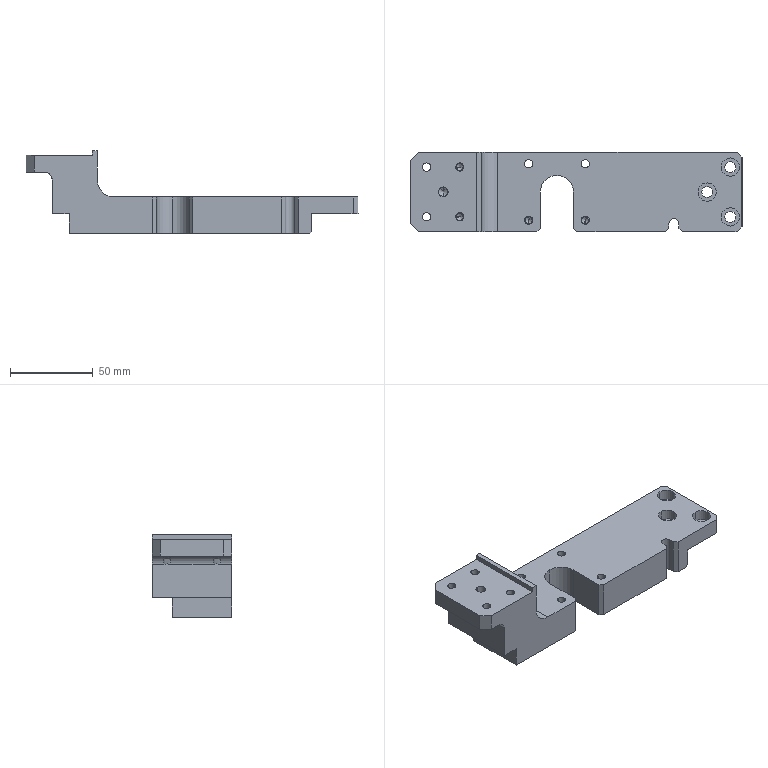Part | STEP file | J454-EBZ05-13-00-Part-1-4 | 1 solid | 119 faces | box 200 x 48 x 50 mm | volume 172584 mm3 | cylinder 59 | plane 42 | cone 16 | spline 2 | commonest cylinder face diameters 5 x22 4.2 x14 6.6 x6 11 x6 6 x3 10 x3